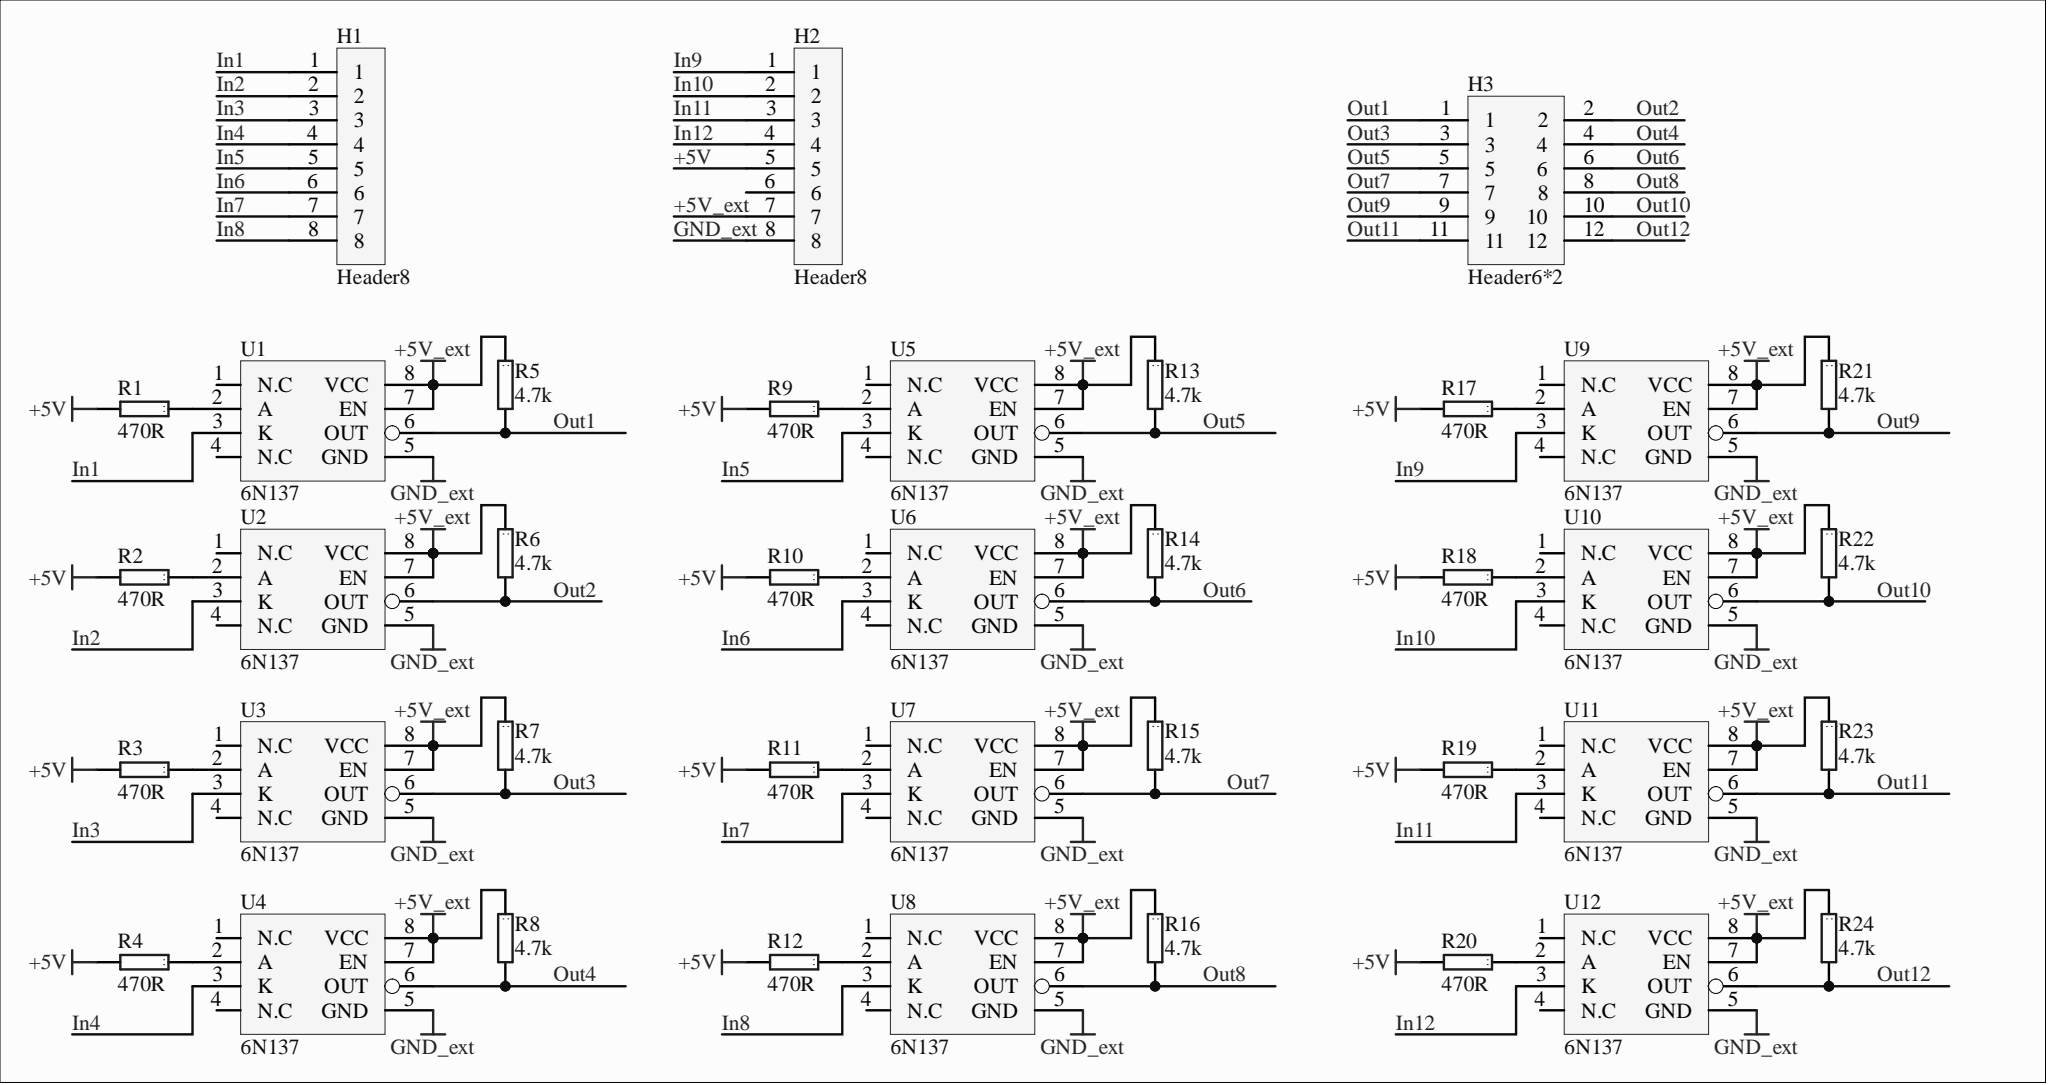Circuit board | Altium Designer | 39 parts | 39 nets
Bill of materials:
Comment,Description,Designator,Footprint,LibRef,Quantity
"Header8","Header8","H1, H2","PinHeader8_1.27mm","Header8","2"
"Header6*2","Header6*2","H3","PinHeader6*2_2.54mm","Header6*2","1"
"470R","","R1, R2, R3, R4, R9, R10, R11, R12, R17, R18, R19, R20","0603","RES","12"
"4.7k","","R5, R6, R7, R8, R13, R14, R15, R16, R21, R22, R23, R24","0603","RES","12"
"6N137","High-speed optocoupler","U1, U2, U3, U4, U5, U6, U7, U8, U9, U10, U11, U12","6N137_SMD","6N137","12"
Netlist (Protel format):
[
H1
PinHeader8_1.27mm
Header8



]
[
H2
PinHeader8_1.27mm
Header8



]
[
H3
PinHeader6*2_2.54mm
Header6*2



]
[
R1
0603
470R



]
[
R2
0603
470R



]
[
R3
0603
470R



]
[
R4
0603
470R



]
[
R5
0603
4.7k



]
[
R6
0603
4.7k



]
[
R7
0603
4.7k



]
[
R8
0603
4.7k



]
[
R9
0603
470R



]
[
R10
0603
470R



]
[
R11
0603
470R



]
[
R12
0603
470R



]
[
R13
0603
4.7k



]
[
R14
0603
4.7k



]
[
R15
0603
4.7k



]
[
R16
0603
4.7k



]
[
R17
0603
470R



]
[
R18
0603
470R



]
[
R19
0603
470R



]
[
R20
0603
470R



]
[
R21
0603
4.7k



]
[
R22
0603
4.7k



]
[
R23
0603
4.7k



]
[
R24
0603
4.7k



]
[
U1
6N137_SMD
6N137



]
[
U2
6N137_SMD
6N137



]
[
U3
6N137_SMD
6N137



]
[
U4
6N137_SMD
6N137



]
[
U5
6N137_SMD
6N137



]
[
U6
6N137_SMD
6N137



]
[
U7
6N137_SMD
6N137



]
[
U8
6N137_SMD
6N137



]
[
U9
6N137_SMD
6N137



]
[
U10
6N137_SMD
6N137



]
[
U11
6N137_SMD
6N137



]
[
U12
6N137_SMD
6N137



]
(
Out12
H3-12
R24-2
U12-6
)
(
Out11
H3-11
R23-2
U11-6
)
(
Out10
H3-10
R22-2
U10-6
)
(
Out9
H3-9
R21-2
U9-6
)
(
Out8
H3-8
R16-2
U8-6
)
(
Out7
H3-7
R15-2
U7-6
)
(
Out6
H3-6
R14-2
U6-6
)
(
Out5
H3-5
R13-2
U5-6
)
(
Out4
H3-4
R8-2
U4-6
)
(
Out3
H3-3
R7-2
U3-6
)
(
Out2
H3-2
R6-2
U2-6
)
(
Out1
H3-1
R5-2
U1-6
)
(
NetR20_1
R20-1
U12-2
)
(
NetR19_1
R19-1
U11-2
)
(
NetR18_1
R18-1
U10-2
)
(
NetR17_1
R17-1
U9-2
)
(
NetR12_1
R12-1
U8-2
)
(
NetR11_1
R11-1
U7-2
)
(
NetR10_1
R10-1
U6-2
)
(
NetR9_1
R9-1
U5-2
)
(
NetR4_1
R4-1
U4-2
)
(
NetR3_1
R3-1
U3-2
)
(
NetR2_1
R2-1
U2-2
)
(
NetR1_1
R1-1
U1-2
)
(
In12
H2-4
U12-3
)
(
In11
H2-3
U11-3
)
(
In10
H2-2
U10-3
)
(
In9
H2-1
U9-3
)
(
In8
H1-8
U8-3
)
(
In7
H1-7
U7-3
)
(
In6
H1-6
U6-3
)
(
In5
H1-5
U5-3
)
(
In4
H1-4
U4-3
)
(
In3
H1-3
U3-3
)
(
In2
H1-2
U2-3
)
(
In1
H1-1
U1-3
)
(
GND_ext
H2-8
U1-5
U2-5
U3-5
U4-5
U5-5
U6-5
U7-5
U8-5
U9-5
U10-5
U11-5
U12-5
)
(
+5V_ext
H2-7
R5-1
R6-1
R7-1
R8-1
R13-1
R14-1
R15-1
R16-1
R21-1
R22-1
R23-1
R24-1
U1-7
U1-8
U2-7
U2-8
U3-7
U3-8
U4-7
U4-8
U5-7
U5-8
U6-7
U6-8
U7-7
U7-8
U8-7
U8-8
U9-7
U9-8
U10-7
U10-8
U11-7
U11-8
U12-7
U12-8
)
(
+5V
H2-5
R1-2
R2-2
R3-2
R4-2
R9-2
R10-2
R11-2
R12-2
R17-2
R18-2
R19-2
R20-2
)